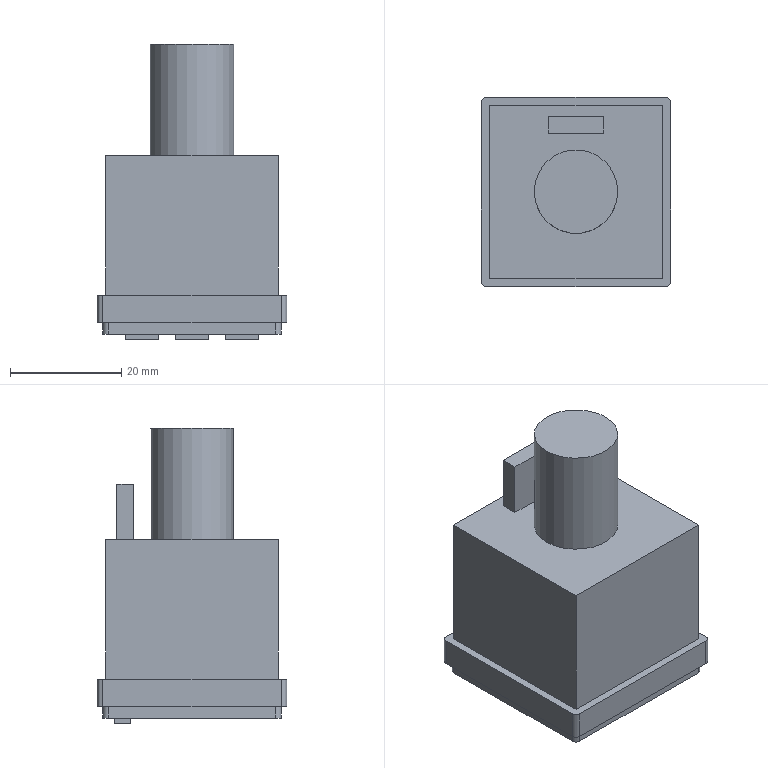Part | NX | 1 solid | 51 faces | box 34 x 34 x 53 mm | volume 35678 mm3 | plane 42 | cylinder 9 | commonest cylinder face diameters 2 x8 15 x1
STEP:
#1=CARTESIAN_POINT('',(-7.5,0.,30.));
#2=VERTEX_POINT('',#1);
#3=CARTESIAN_POINT('',(0.,0.,30.));
#4=DIRECTION('',(0.,0.,-1.));
#5=DIRECTION('',(-1.,0.,0.));
#6=AXIS2_PLACEMENT_3D('',#3,#4,#5);
#7=CIRCLE('',#6,7.5);
#8=EDGE_CURVE('',#2,#2,#7,.F.);
#9=ORIENTED_EDGE('',*,*,#8,.F.);
#10=EDGE_LOOP('',(#9));
#11=FACE_BOUND('',#10,.T.);
#12=CARTESIAN_POINT('',(-15.5,15.5,30.));
#13=VERTEX_POINT('',#12);
#14=CARTESIAN_POINT('',(-15.5,-15.5,30.));
#15=VERTEX_POINT('',#14);
#16=CARTESIAN_POINT('',(-15.5,15.5,30.));
#17=DIRECTION('',(0.,-1.,0.));
#18=VECTOR('',#17,1000.);
#19=LINE('',#16,#18);
#20=EDGE_CURVE('',#13,#15,#19,.T.);
#21=ORIENTED_EDGE('',*,*,#20,.T.);
#22=CARTESIAN_POINT('',(15.5,-15.5,30.));
#23=VERTEX_POINT('',#22);
#24=CARTESIAN_POINT('',(15.5,-15.5,30.));
#25=DIRECTION('',(1.,0.,0.));
#26=VECTOR('',#25,1000.);
#27=LINE('',#24,#26);
#28=EDGE_CURVE('',#15,#23,#27,.T.);
#29=ORIENTED_EDGE('',*,*,#28,.T.);
#30=CARTESIAN_POINT('',(15.5,15.5,30.));
#31=VERTEX_POINT('',#30);
#32=CARTESIAN_POINT('',(15.5,15.5,30.));
#33=DIRECTION('',(0.,1.,0.));
#34=VECTOR('',#33,1000.);
#35=LINE('',#32,#34);
#36=EDGE_CURVE('',#23,#31,#35,.T.);
#37=ORIENTED_EDGE('',*,*,#36,.T.);
#38=CARTESIAN_POINT('',(15.5,15.5,30.));
#39=DIRECTION('',(-1.,0.,0.));
#40=VECTOR('',#39,1000.);
#41=LINE('',#38,#40);
#42=EDGE_CURVE('',#31,#13,#41,.T.);
#43=ORIENTED_EDGE('',*,*,#42,.T.);
#44=EDGE_LOOP('',(#21,#29,#37,#43));
#45=FACE_BOUND('',#44,.T.);
#46=CARTESIAN_POINT('',(5.,10.5,30.));
#47=VERTEX_POINT('',#46);
#48=CARTESIAN_POINT('',(5.,13.5,30.));
#49=VERTEX_POINT('',#48);
#50=CARTESIAN_POINT('',(5.,13.5,30.));
#51=DIRECTION('',(0.,1.,0.));
#52=VECTOR('',#51,1000.);
#53=LINE('',#50,#52);
#54=EDGE_CURVE('',#47,#49,#53,.T.);
#55=ORIENTED_EDGE('',*,*,#54,.F.);
#56=CARTESIAN_POINT('',(-5.,10.5,30.));
#57=VERTEX_POINT('',#56);
#58=CARTESIAN_POINT('',(5.,10.5,30.));
#59=DIRECTION('',(1.,0.,0.));
#60=VECTOR('',#59,1000.);
#61=LINE('',#58,#60);
#62=EDGE_CURVE('',#57,#47,#61,.T.);
#63=ORIENTED_EDGE('',*,*,#62,.F.);
#64=CARTESIAN_POINT('',(-5.,13.5,30.));
#65=VERTEX_POINT('',#64);
#66=CARTESIAN_POINT('',(-5.,13.5,30.));
#67=DIRECTION('',(0.,-1.,0.));
#68=VECTOR('',#67,1000.);
#69=LINE('',#66,#68);
#70=EDGE_CURVE('',#65,#57,#69,.T.);
#71=ORIENTED_EDGE('',*,*,#70,.F.);
#72=CARTESIAN_POINT('',(5.,13.5,30.));
#73=DIRECTION('',(-1.,0.,0.));
#74=VECTOR('',#73,1000.);
#75=LINE('',#72,#74);
#76=EDGE_CURVE('',#49,#65,#75,.T.);
#77=ORIENTED_EDGE('',*,*,#76,.F.);
#78=EDGE_LOOP('',(#55,#63,#71,#77));
#79=FACE_BOUND('',#78,.T.);
#80=CARTESIAN_POINT('',(0.,0.,30.));
#81=DIRECTION('',(0.,0.,-1.));
#82=DIRECTION('',(-1.,0.,0.));
#83=AXIS2_PLACEMENT_3D('',#80,#81,#82);
#84=PLANE('',#83);
#85=ADVANCED_FACE('',(#11,#45,#79),#84,.F.);
#86=CARTESIAN_POINT('',(13.,8.5,-2.));
#87=VERTEX_POINT('',#86);
#88=CARTESIAN_POINT('',(13.,-13.5,-2.));
#89=VERTEX_POINT('',#88);
#90=CARTESIAN_POINT('',(13.,8.5,-2.));
#91=DIRECTION('',(0.,-1.,0.));
#92=VECTOR('',#91,1000.);
#93=LINE('',#90,#92);
#94=EDGE_CURVE('',#87,#89,#93,.T.);
#95=ORIENTED_EDGE('',*,*,#94,.F.);
#96=CARTESIAN_POINT('',(-13.,8.5,-2.));
#97=VERTEX_POINT('',#96);
#98=CARTESIAN_POINT('',(-13.,8.5,-2.));
#99=DIRECTION('',(1.,0.,0.));
#100=VECTOR('',#99,1000.);
#101=LINE('',#98,#100);
#102=EDGE_CURVE('',#97,#87,#101,.T.);
#103=ORIENTED_EDGE('',*,*,#102,.F.);
#104=CARTESIAN_POINT('',(-13.,-13.5,-2.));
#105=VERTEX_POINT('',#104);
#106=CARTESIAN_POINT('',(-13.,8.5,-2.));
#107=DIRECTION('',(0.,1.,0.));
#108=VECTOR('',#107,1000.);
#109=LINE('',#106,#108);
#110=EDGE_CURVE('',#105,#97,#109,.T.);
#111=ORIENTED_EDGE('',*,*,#110,.F.);
#112=CARTESIAN_POINT('',(-13.,-13.5,-2.));
#113=DIRECTION('',(-1.,0.,0.));
#114=VECTOR('',#113,1000.);
#115=LINE('',#112,#114);
#116=EDGE_CURVE('',#89,#105,#115,.T.);
#117=ORIENTED_EDGE('',*,*,#116,.F.);
#118=EDGE_LOOP('',(#95,#103,#111,#117));
#119=FACE_BOUND('',#118,.T.);
#120=CARTESIAN_POINT('',(3.,11.,-2.));
#121=VERTEX_POINT('',#120);
#122=CARTESIAN_POINT('',(-3.,11.,-2.));
#123=VERTEX_POINT('',#122);
#124=CARTESIAN_POINT('',(3.,11.,-2.));
#125=DIRECTION('',(-1.,0.,0.));
#126=VECTOR('',#125,1000.);
#127=LINE('',#124,#126);
#128=EDGE_CURVE('',#121,#123,#127,.T.);
#129=ORIENTED_EDGE('',*,*,#128,.F.);
#130=CARTESIAN_POINT('',(3.,14.,-2.));
#131=VERTEX_POINT('',#130);
#132=CARTESIAN_POINT('',(3.,14.,-2.));
#133=DIRECTION('',(0.,-1.,0.));
#134=VECTOR('',#133,1000.);
#135=LINE('',#132,#134);
#136=EDGE_CURVE('',#131,#121,#135,.T.);
#137=ORIENTED_EDGE('',*,*,#136,.F.);
#138=CARTESIAN_POINT('',(-3.,14.,-2.));
#139=VERTEX_POINT('',#138);
#140=CARTESIAN_POINT('',(3.,14.,-2.));
#141=DIRECTION('',(1.,0.,0.));
#142=VECTOR('',#141,1000.);
#143=LINE('',#140,#142);
#144=EDGE_CURVE('',#139,#131,#143,.T.);
#145=ORIENTED_EDGE('',*,*,#144,.F.);
#146=CARTESIAN_POINT('',(-3.,14.,-2.));
#147=DIRECTION('',(0.,1.,0.));
#148=VECTOR('',#147,1000.);
#149=LINE('',#146,#148);
#150=EDGE_CURVE('',#123,#139,#149,.T.);
#151=ORIENTED_EDGE('',*,*,#150,.F.);
#152=EDGE_LOOP('',(#129,#137,#145,#151));
#153=FACE_BOUND('',#152,.T.);
#154=CARTESIAN_POINT('',(-15.,16.,-2.));
#155=VERTEX_POINT('',#154);
#156=CARTESIAN_POINT('',(15.,16.,-2.));
#157=VERTEX_POINT('',#156);
#158=CARTESIAN_POINT('',(-16.,16.,-2.));
#159=DIRECTION('',(1.,0.,0.));
#160=VECTOR('',#159,1000.);
#161=LINE('',#158,#160);
#162=EDGE_CURVE('',#155,#157,#161,.T.);
#163=ORIENTED_EDGE('',*,*,#162,.T.);
#164=CARTESIAN_POINT('',(16.,15.,-2.));
#165=VERTEX_POINT('',#164);
#166=CARTESIAN_POINT('',(15.,15.,-2.));
#167=DIRECTION('',(0.,0.,-1.));
#168=DIRECTION('',(-1.,0.,0.));
#169=AXIS2_PLACEMENT_3D('',#166,#167,#168);
#170=CIRCLE('',#169,1.);
#171=EDGE_CURVE('',#157,#165,#170,.T.);
#172=ORIENTED_EDGE('',*,*,#171,.T.);
#173=CARTESIAN_POINT('',(16.,-15.,-2.));
#174=VERTEX_POINT('',#173);
#175=CARTESIAN_POINT('',(16.,16.,-2.));
#176=DIRECTION('',(0.,-1.,0.));
#177=VECTOR('',#176,1000.);
#178=LINE('',#175,#177);
#179=EDGE_CURVE('',#165,#174,#178,.T.);
#180=ORIENTED_EDGE('',*,*,#179,.T.);
#181=CARTESIAN_POINT('',(15.,-16.,-2.));
#182=VERTEX_POINT('',#181);
#183=CARTESIAN_POINT('',(15.,-15.,-2.));
#184=DIRECTION('',(0.,0.,-1.));
#185=DIRECTION('',(-1.,0.,0.));
#186=AXIS2_PLACEMENT_3D('',#183,#184,#185);
#187=CIRCLE('',#186,1.);
#188=EDGE_CURVE('',#174,#182,#187,.T.);
#189=ORIENTED_EDGE('',*,*,#188,.T.);
#190=CARTESIAN_POINT('',(-15.,-16.,-2.));
#191=VERTEX_POINT('',#190);
#192=CARTESIAN_POINT('',(16.,-16.,-2.));
#193=DIRECTION('',(-1.,0.,0.));
#194=VECTOR('',#193,1000.);
#195=LINE('',#192,#194);
#196=EDGE_CURVE('',#182,#191,#195,.T.);
#197=ORIENTED_EDGE('',*,*,#196,.T.);
#198=CARTESIAN_POINT('',(-16.,-15.,-2.));
#199=VERTEX_POINT('',#198);
#200=CARTESIAN_POINT('',(-15.,-15.,-2.));
#201=DIRECTION('',(0.,0.,-1.));
#202=DIRECTION('',(-1.,0.,0.));
#203=AXIS2_PLACEMENT_3D('',#200,#201,#202);
#204=CIRCLE('',#203,1.);
#205=EDGE_CURVE('',#191,#199,#204,.T.);
#206=ORIENTED_EDGE('',*,*,#205,.T.);
#207=CARTESIAN_POINT('',(-16.,15.,-2.));
#208=VERTEX_POINT('',#207);
#209=CARTESIAN_POINT('',(-16.,-16.,-2.));
#210=DIRECTION('',(0.,1.,0.));
#211=VECTOR('',#210,1000.);
#212=LINE('',#209,#211);
#213=EDGE_CURVE('',#199,#208,#212,.T.);
#214=ORIENTED_EDGE('',*,*,#213,.T.);
#215=CARTESIAN_POINT('',(-15.,15.,-2.));
#216=DIRECTION('',(0.,0.,-1.));
#217=DIRECTION('',(-1.,0.,0.));
#218=AXIS2_PLACEMENT_3D('',#215,#216,#217);
#219=CIRCLE('',#218,1.);
#220=EDGE_CURVE('',#208,#155,#219,.T.);
#221=ORIENTED_EDGE('',*,*,#220,.T.);
#222=EDGE_LOOP('',(#163,#172,#180,#189,#197,#206,#214,#221));
#223=FACE_BOUND('',#222,.T.);
#224=CARTESIAN_POINT('',(12.,11.,-2.));
#225=VERTEX_POINT('',#224);
#226=CARTESIAN_POINT('',(6.,11.,-2.));
#227=VERTEX_POINT('',#226);
#228=CARTESIAN_POINT('',(12.,11.,-2.));
#229=DIRECTION('',(-1.,0.,0.));
#230=VECTOR('',#229,1000.);
#231=LINE('',#228,#230);
#232=EDGE_CURVE('',#225,#227,#231,.T.);
#233=ORIENTED_EDGE('',*,*,#232,.F.);
#234=CARTESIAN_POINT('',(12.,14.,-2.));
#235=VERTEX_POINT('',#234);
#236=CARTESIAN_POINT('',(12.,14.,-2.));
#237=DIRECTION('',(0.,-1.,0.));
#238=VECTOR('',#237,1000.);
#239=LINE('',#236,#238);
#240=EDGE_CURVE('',#235,#225,#239,.T.);
#241=ORIENTED_EDGE('',*,*,#240,.F.);
#242=CARTESIAN_POINT('',(6.,14.,-2.));
#243=VERTEX_POINT('',#242);
#244=CARTESIAN_POINT('',(12.,14.,-2.));
#245=DIRECTION('',(1.,0.,0.));
#246=VECTOR('',#245,1000.);
#247=LINE('',#244,#246);
#248=EDGE_CURVE('',#243,#235,#247,.T.);
#249=ORIENTED_EDGE('',*,*,#248,.F.);
#250=CARTESIAN_POINT('',(6.,14.,-2.));
#251=DIRECTION('',(0.,1.,0.));
#252=VECTOR('',#251,1000.);
#253=LINE('',#250,#252);
#254=EDGE_CURVE('',#227,#243,#253,.T.);
#255=ORIENTED_EDGE('',*,*,#254,.F.);
#256=EDGE_LOOP('',(#233,#241,#249,#255));
#257=FACE_BOUND('',#256,.T.);
#258=CARTESIAN_POINT('',(-6.,11.,-2.));
#259=VERTEX_POINT('',#258);
#260=CARTESIAN_POINT('',(-12.,11.,-2.));
#261=VERTEX_POINT('',#260);
#262=CARTESIAN_POINT('',(-6.,11.,-2.));
#263=DIRECTION('',(-1.,0.,0.));
#264=VECTOR('',#263,1000.);
#265=LINE('',#262,#264);
#266=EDGE_CURVE('',#259,#261,#265,.T.);
#267=ORIENTED_EDGE('',*,*,#266,.F.);
#268=CARTESIAN_POINT('',(-6.,14.,-2.));
#269=VERTEX_POINT('',#268);
#270=CARTESIAN_POINT('',(-6.,14.,-2.));
#271=DIRECTION('',(0.,-1.,0.));
#272=VECTOR('',#271,1000.);
#273=LINE('',#270,#272);
#274=EDGE_CURVE('',#269,#259,#273,.T.);
#275=ORIENTED_EDGE('',*,*,#274,.F.);
#276=CARTESIAN_POINT('',(-12.,14.,-2.));
#277=VERTEX_POINT('',#276);
#278=CARTESIAN_POINT('',(-6.,14.,-2.));
#279=DIRECTION('',(1.,0.,0.));
#280=VECTOR('',#279,1000.);
#281=LINE('',#278,#280);
#282=EDGE_CURVE('',#277,#269,#281,.T.);
#283=ORIENTED_EDGE('',*,*,#282,.F.);
#284=CARTESIAN_POINT('',(-12.,14.,-2.));
#285=DIRECTION('',(0.,1.,0.));
#286=VECTOR('',#285,1000.);
#287=LINE('',#284,#286);
#288=EDGE_CURVE('',#261,#277,#287,.T.);
#289=ORIENTED_EDGE('',*,*,#288,.F.);
#290=EDGE_LOOP('',(#267,#275,#283,#289));
#291=FACE_BOUND('',#290,.T.);
#292=CARTESIAN_POINT('',(0.,0.,-2.));
#293=DIRECTION('',(0.,0.,-1.));
#294=DIRECTION('',(-1.,0.,0.));
#295=AXIS2_PLACEMENT_3D('',#292,#293,#294);
#296=PLANE('',#295);
#297=ADVANCED_FACE('',(#119,#153,#223,#257,#291),#296,.T.);
#298=CARTESIAN_POINT('',(16.,17.,0.));
#299=VERTEX_POINT('',#298);
#300=CARTESIAN_POINT('',(-16.,17.,0.));
#301=VERTEX_POINT('',#300);
#302=CARTESIAN_POINT('',(-17.,17.,0.));
#303=DIRECTION('',(-1.,0.,0.));
#304=VECTOR('',#303,1000.);
#305=LINE('',#302,#304);
#306=EDGE_CURVE('',#299,#301,#305,.T.);
#307=ORIENTED_EDGE('',*,*,#306,.F.);
#308=CARTESIAN_POINT('',(17.,16.,0.));
#309=VERTEX_POINT('',#308);
#310=CARTESIAN_POINT('',(16.,16.,0.));
#311=DIRECTION('',(0.,0.,1.));
#312=DIRECTION('',(1.,0.,0.));
#313=AXIS2_PLACEMENT_3D('',#310,#311,#312);
#314=CIRCLE('',#313,1.);
#315=EDGE_CURVE('',#299,#309,#314,.F.);
#316=ORIENTED_EDGE('',*,*,#315,.T.);
#317=CARTESIAN_POINT('',(17.,-16.,0.));
#318=VERTEX_POINT('',#317);
#319=CARTESIAN_POINT('',(17.,17.,0.));
#320=DIRECTION('',(0.,1.,0.));
#321=VECTOR('',#320,1000.);
#322=LINE('',#319,#321);
#323=EDGE_CURVE('',#318,#309,#322,.T.);
#324=ORIENTED_EDGE('',*,*,#323,.F.);
#325=CARTESIAN_POINT('',(16.,-17.,0.));
#326=VERTEX_POINT('',#325);
#327=CARTESIAN_POINT('',(16.,-16.,0.));
#328=DIRECTION('',(0.,0.,1.));
#329=DIRECTION('',(1.,0.,0.));
#330=AXIS2_PLACEMENT_3D('',#327,#328,#329);
#331=CIRCLE('',#330,1.);
#332=EDGE_CURVE('',#318,#326,#331,.F.);
#333=ORIENTED_EDGE('',*,*,#332,.T.);
#334=CARTESIAN_POINT('',(-16.,-17.,0.));
#335=VERTEX_POINT('',#334);
#336=CARTESIAN_POINT('',(-17.,-17.,0.));
#337=DIRECTION('',(1.,0.,0.));
#338=VECTOR('',#337,1000.);
#339=LINE('',#336,#338);
#340=EDGE_CURVE('',#335,#326,#339,.T.);
#341=ORIENTED_EDGE('',*,*,#340,.F.);
#342=CARTESIAN_POINT('',(-17.,-16.,0.));
#343=VERTEX_POINT('',#342);
#344=CARTESIAN_POINT('',(-16.,-16.,0.));
#345=DIRECTION('',(0.,0.,1.));
#346=DIRECTION('',(1.,0.,0.));
#347=AXIS2_PLACEMENT_3D('',#344,#345,#346);
#348=CIRCLE('',#347,1.);
#349=EDGE_CURVE('',#335,#343,#348,.F.);
#350=ORIENTED_EDGE('',*,*,#349,.T.);
#351=CARTESIAN_POINT('',(-17.,16.,0.));
#352=VERTEX_POINT('',#351);
#353=CARTESIAN_POINT('',(-17.,17.,0.));
#354=DIRECTION('',(0.,-1.,0.));
#355=VECTOR('',#354,1000.);
#356=LINE('',#353,#355);
#357=EDGE_CURVE('',#352,#343,#356,.T.);
#358=ORIENTED_EDGE('',*,*,#357,.F.);
#359=CARTESIAN_POINT('',(-16.,16.,0.));
#360=DIRECTION('',(0.,0.,1.));
#361=DIRECTION('',(1.,0.,0.));
#362=AXIS2_PLACEMENT_3D('',#359,#360,#361);
#363=CIRCLE('',#362,1.);
#364=EDGE_CURVE('',#352,#301,#363,.F.);
#365=ORIENTED_EDGE('',*,*,#364,.T.);
#366=EDGE_LOOP('',(#307,#316,#324,#333,#341,#350,#358,#365));
#367=FACE_BOUND('',#366,.T.);
#368=CARTESIAN_POINT('',(-15.,16.,0.));
#369=VERTEX_POINT('',#368);
#370=CARTESIAN_POINT('',(15.,16.,0.));
#371=VERTEX_POINT('',#370);
#372=CARTESIAN_POINT('',(-16.,16.,0.));
#373=DIRECTION('',(1.,0.,0.));
#374=VECTOR('',#373,1000.);
#375=LINE('',#372,#374);
#376=EDGE_CURVE('',#369,#371,#375,.T.);
#377=ORIENTED_EDGE('',*,*,#376,.F.);
#378=CARTESIAN_POINT('',(-16.,15.,0.));
#379=VERTEX_POINT('',#378);
#380=CARTESIAN_POINT('',(-15.,15.,0.));
#381=DIRECTION('',(0.,0.,1.));
#382=DIRECTION('',(1.,0.,0.));
#383=AXIS2_PLACEMENT_3D('',#380,#381,#382);
#384=CIRCLE('',#383,1.);
#385=EDGE_CURVE('',#369,#379,#384,.T.);
#386=ORIENTED_EDGE('',*,*,#385,.T.);
#387=CARTESIAN_POINT('',(-16.,-15.,0.));
#388=VERTEX_POINT('',#387);
#389=CARTESIAN_POINT('',(-16.,-16.,0.));
#390=DIRECTION('',(0.,1.,0.));
#391=VECTOR('',#390,1000.);
#392=LINE('',#389,#391);
#393=EDGE_CURVE('',#388,#379,#392,.T.);
#394=ORIENTED_EDGE('',*,*,#393,.F.);
#395=CARTESIAN_POINT('',(-15.,-16.,0.));
#396=VERTEX_POINT('',#395);
#397=CARTESIAN_POINT('',(-15.,-15.,0.));
#398=DIRECTION('',(0.,0.,1.));
#399=DIRECTION('',(1.,0.,0.));
#400=AXIS2_PLACEMENT_3D('',#397,#398,#399);
#401=CIRCLE('',#400,1.);
#402=EDGE_CURVE('',#388,#396,#401,.T.);
#403=ORIENTED_EDGE('',*,*,#402,.T.);
#404=CARTESIAN_POINT('',(15.,-16.,0.));
#405=VERTEX_POINT('',#404);
#406=CARTESIAN_POINT('',(16.,-16.,0.));
#407=DIRECTION('',(-1.,0.,0.));
#408=VECTOR('',#407,1000.);
#409=LINE('',#406,#408);
#410=EDGE_CURVE('',#405,#396,#409,.T.);
#411=ORIENTED_EDGE('',*,*,#410,.F.);
#412=CARTESIAN_POINT('',(16.,-15.,0.));
#413=VERTEX_POINT('',#412);
#414=CARTESIAN_POINT('',(15.,-15.,0.));
#415=DIRECTION('',(0.,0.,1.));
#416=DIRECTION('',(1.,0.,0.));
#417=AXIS2_PLACEMENT_3D('',#414,#415,#416);
#418=CIRCLE('',#417,1.);
#419=EDGE_CURVE('',#405,#413,#418,.T.);
#420=ORIENTED_EDGE('',*,*,#419,.T.);
#421=CARTESIAN_POINT('',(16.,15.,0.));
#422=VERTEX_POINT('',#421);
#423=CARTESIAN_POINT('',(16.,16.,0.));
#424=DIRECTION('',(0.,-1.,0.));
#425=VECTOR('',#424,1000.);
#426=LINE('',#423,#425);
#427=EDGE_CURVE('',#422,#413,#426,.T.);
#428=ORIENTED_EDGE('',*,*,#427,.F.);
#429=CARTESIAN_POINT('',(15.,15.,0.));
#430=DIRECTION('',(0.,0.,1.));
#431=DIRECTION('',(1.,0.,0.));
#432=AXIS2_PLACEMENT_3D('',#429,#430,#431);
#433=CIRCLE('',#432,1.);
#434=EDGE_CURVE('',#422,#371,#433,.T.);
#435=ORIENTED_EDGE('',*,*,#434,.T.);
#436=EDGE_LOOP('',(#377,#386,#394,#403,#411,#420,#428,#435));
#437=FACE_BOUND('',#436,.T.);
#438=CARTESIAN_POINT('',(0.,0.,0.));
#439=DIRECTION('',(0.,0.,1.));
#440=DIRECTION('',(1.,0.,0.));
#441=AXIS2_PLACEMENT_3D('',#438,#439,#440);
#442=PLANE('',#441);
#443=ADVANCED_FACE('',(#367,#437),#442,.F.);
#444=CARTESIAN_POINT('',(17.,-16.,5.));
#445=VERTEX_POINT('',#444);
#446=CARTESIAN_POINT('',(17.,16.,5.));
#447=VERTEX_POINT('',#446);
#448=CARTESIAN_POINT('',(17.,17.,5.));
#449=DIRECTION('',(0.,1.,0.));
#450=VECTOR('',#449,1000.);
#451=LINE('',#448,#450);
#452=EDGE_CURVE('',#445,#447,#451,.T.);
#453=ORIENTED_EDGE('',*,*,#452,.T.);
#454=CARTESIAN_POINT('',(16.,17.,5.));
#455=VERTEX_POINT('',#454);
#456=CARTESIAN_POINT('',(16.,16.,5.));
#457=DIRECTION('',(0.,0.,1.));
#458=DIRECTION('',(1.,0.,0.));
#459=AXIS2_PLACEMENT_3D('',#456,#457,#458);
#460=CIRCLE('',#459,1.);
#461=EDGE_CURVE('',#447,#455,#460,.T.);
#462=ORIENTED_EDGE('',*,*,#461,.T.);
#463=CARTESIAN_POINT('',(-16.,17.,5.));
#464=VERTEX_POINT('',#463);
#465=CARTESIAN_POINT('',(-17.,17.,5.));
#466=DIRECTION('',(-1.,0.,0.));
#467=VECTOR('',#466,1000.);
#468=LINE('',#465,#467);
#469=EDGE_CURVE('',#455,#464,#468,.T.);
#470=ORIENTED_EDGE('',*,*,#469,.T.);
#471=CARTESIAN_POINT('',(-17.,16.,5.));
#472=VERTEX_POINT('',#471);
#473=CARTESIAN_POINT('',(-16.,16.,5.));
#474=DIRECTION('',(0.,0.,1.));
#475=DIRECTION('',(1.,0.,0.));
#476=AXIS2_PLACEMENT_3D('',#473,#474,#475);
#477=CIRCLE('',#476,1.);
#478=EDGE_CURVE('',#464,#472,#477,.T.);
#479=ORIENTED_EDGE('',*,*,#478,.T.);
#480=CARTESIAN_POINT('',(-17.,-16.,5.));
#481=VERTEX_POINT('',#480);
#482=CARTESIAN_POINT('',(-17.,17.,5.));
#483=DIRECTION('',(0.,-1.,0.));
#484=VECTOR('',#483,1000.);
#485=LINE('',#482,#484);
#486=EDGE_CURVE('',#472,#481,#485,.T.);
#487=ORIENTED_EDGE('',*,*,#486,.T.);
#488=CARTESIAN_POINT('',(-16.,-17.,5.));
#489=VERTEX_POINT('',#488);
#490=CARTESIAN_POINT('',(-16.,-16.,5.));
#491=DIRECTION('',(0.,0.,1.));
#492=DIRECTION('',(1.,0.,0.));
#493=AXIS2_PLACEMENT_3D('',#490,#491,#492);
#494=CIRCLE('',#493,1.);
#495=EDGE_CURVE('',#481,#489,#494,.T.);
#496=ORIENTED_EDGE('',*,*,#495,.T.);
#497=CARTESIAN_POINT('',(16.,-17.,5.));
#498=VERTEX_POINT('',#497);
#499=CARTESIAN_POINT('',(-17.,-17.,5.));
#500=DIRECTION('',(1.,0.,0.));
#501=VECTOR('',#500,1000.);
#502=LINE('',#499,#501);
#503=EDGE_CURVE('',#489,#498,#502,.T.);
#504=ORIENTED_EDGE('',*,*,#503,.T.);
#505=CARTESIAN_POINT('',(16.,-16.,5.));
#506=DIRECTION('',(0.,0.,1.));
#507=DIRECTION('',(1.,0.,0.));
#508=AXIS2_PLACEMENT_3D('',#505,#506,#507);
#509=CIRCLE('',#508,1.);
#510=EDGE_CURVE('',#498,#445,#509,.T.);
#511=ORIENTED_EDGE('',*,*,#510,.T.);
#512=EDGE_LOOP('',(#453,#462,#470,#479,#487,#496,#504,#511));
#513=FACE_BOUND('',#512,.T.);
#514=CARTESIAN_POINT('',(-15.5,-15.5,5.));
#515=VERTEX_POINT('',#514);
#516=CARTESIAN_POINT('',(15.5,-15.5,5.));
#517=VERTEX_POINT('',#516);
#518=CARTESIAN_POINT('',(15.5,-15.5,5.));
#519=DIRECTION('',(1.,0.,0.));
#520=VECTOR('',#519,1000.);
#521=LINE('',#518,#520);
#522=EDGE_CURVE('',#515,#517,#521,.T.);
#523=ORIENTED_EDGE('',*,*,#522,.F.);
#524=CARTESIAN_POINT('',(-15.5,15.5,5.));
#525=VERTEX_POINT('',#524);
#526=CARTESIAN_POINT('',(-15.5,15.5,5.));
#527=DIRECTION('',(0.,-1.,0.));
#528=VECTOR('',#527,1000.);
#529=LINE('',#526,#528);
#530=EDGE_CURVE('',#525,#515,#529,.T.);
#531=ORIENTED_EDGE('',*,*,#530,.F.);
#532=CARTESIAN_POINT('',(15.5,15.5,5.));
#533=VERTEX_POINT('',#532);
#534=CARTESIAN_POINT('',(15.5,15.5,5.));
#535=DIRECTION('',(-1.,0.,0.));
#536=VECTOR('',#535,1000.);
#537=LINE('',#534,#536);
#538=EDGE_CURVE('',#533,#525,#537,.T.);
#539=ORIENTED_EDGE('',*,*,#538,.F.);
#540=CARTESIAN_POINT('',(15.5,15.5,5.));
#541=DIRECTION('',(0.,1.,0.));
#542=VECTOR('',#541,1000.);
#543=LINE('',#540,#542);
#544=EDGE_CURVE('',#517,#533,#543,.T.);
#545=ORIENTED_EDGE('',*,*,#544,.F.);
#546=EDGE_LOOP('',(#523,#531,#539,#545));
#547=FACE_BOUND('',#546,.T.);
#548=CARTESIAN_POINT('',(0.,0.,5.));
#549=DIRECTION('',(0.,0.,1.));
#550=DIRECTION('',(1.,0.,0.));
#551=AXIS2_PLACEMENT_3D('',#548,#549,#550);
#552=PLANE('',#551);
#553=ADVANCED_FACE('',(#513,#547),#552,.T.);
#554=ORIENTED_EDGE('',*,*,#323,.T.);
#555=CARTESIAN_POINT('',(17.,16.,5.));
#556=DIRECTION('',(0.,0.,-1.));
#557=VECTOR('',#556,1000.);
#558=LINE('',#555,#557);
#559=EDGE_CURVE('',#309,#447,#558,.F.);
#560=ORIENTED_EDGE('',*,*,#559,.T.);
#561=ORIENTED_EDGE('',*,*,#452,.F.);
#562=CARTESIAN_POINT('',(17.,-16.,5.));
#563=DIRECTION('',(0.,0.,-1.));
#564=VECTOR('',#563,1000.);
#565=LINE('',#562,#564);
#566=EDGE_CURVE('',#445,#318,#565,.T.);
#567=ORIENTED_EDGE('',*,*,#566,.T.);
#568=EDGE_LOOP('',(#554,#560,#561,#567));
#569=FACE_BOUND('',#568,.T.);
#570=CARTESIAN_POINT('',(17.,17.,5.));
#571=DIRECTION('',(-1.,0.,0.));
#572=DIRECTION('',(0.,-1.,0.));
#573=AXIS2_PLACEMENT_3D('',#570,#571,#572);
#574=PLANE('',#573);
#575=ADVANCED_FACE('',(#569),#574,.F.);
#576=ORIENTED_EDGE('',*,*,#469,.F.);
#577=CARTESIAN_POINT('',(16.,17.,5.));
#578=DIRECTION('',(0.,0.,-1.));
#579=VECTOR('',#578,1000.);
#580=LINE('',#577,#579);
#581=EDGE_CURVE('',#455,#299,#580,.T.);
#582=ORIENTED_EDGE('',*,*,#581,.T.);
#583=ORIENTED_EDGE('',*,*,#306,.T.);
#584=CARTESIAN_POINT('',(-16.,17.,5.));
#585=DIRECTION('',(0.,0.,-1.));
#586=VECTOR('',#585,1000.);
#587=LINE('',#584,#586);
#588=EDGE_CURVE('',#301,#464,#587,.F.);
#589=ORIENTED_EDGE('',*,*,#588,.T.);
#590=EDGE_LOOP('',(#576,#582,#583,#589));
#591=FACE_BOUND('',#590,.T.);
#592=CARTESIAN_POINT('',(-17.,17.,5.));
#593=DIRECTION('',(0.,-1.,0.));
#594=DIRECTION('',(0.,0.,-1.));
#595=AXIS2_PLACEMENT_3D('',#592,#593,#594);
#596=PLANE('',#595);
#597=ADVANCED_FACE('',(#591),#596,.F.);
#598=ORIENTED_EDGE('',*,*,#486,.F.);
#599=CARTESIAN_POINT('',(-17.,16.,5.));
#600=DIRECTION('',(0.,0.,-1.));
#601=VECTOR('',#600,1000.);
#602=LINE('',#599,#601);
#603=EDGE_CURVE('',#472,#352,#602,.T.);
#604=ORIENTED_EDGE('',*,*,#603,.T.);
#605=ORIENTED_EDGE('',*,*,#357,.T.);
#606=CARTESIAN_POINT('',(-17.,-16.,5.));
#607=DIRECTION('',(0.,0.,-1.));
#608=VECTOR('',#607,1000.);
#609=LINE('',#606,#608);
#610=EDGE_CURVE('',#343,#481,#609,.F.);
#611=ORIENTED_EDGE('',*,*,#610,.T.);
#612=EDGE_LOOP('',(#598,#604,#605,#611));
#613=FACE_BOUND('',#612,.T.);
#614=CARTESIAN_POINT('',(-17.,17.,5.));
#615=DIRECTION('',(1.,0.,0.));
#616=DIRECTION('',(0.,1.,0.));
#617=AXIS2_PLACEMENT_3D('',#614,#615,#616);
#618=PLANE('',#617);
#619=ADVANCED_FACE('',(#613),#618,.F.);
#620=ORIENTED_EDGE('',*,*,#503,.F.);
#621=CARTESIAN_POINT('',(-16.,-17.,5.));
#622=DIRECTION('',(0.,0.,-1.));
#623=VECTOR('',#622,1000.);
#624=LINE('',#621,#623);
#625=EDGE_CURVE('',#489,#335,#624,.T.);
#626=ORIENTED_EDGE('',*,*,#625,.T.);
#627=ORIENTED_EDGE('',*,*,#340,.T.);
#628=CARTESIAN_POINT('',(16.,-17.,5.));
#629=DIRECTION('',(0.,0.,-1.));
#630=VECTOR('',#629,1000.);
#631=LINE('',#628,#630);
#632=EDGE_CURVE('',#326,#498,#631,.F.);
#633=ORIENTED_EDGE('',*,*,#632,.T.);
#634=EDGE_LOOP('',(#620,#626,#627,#633));
#635=FACE_BOUND('',#634,.T.);
#636=CARTESIAN_POINT('',(-17.,-17.,5.));
#637=DIRECTION('',(0.,1.,0.));
#638=DIRECTION('',(0.,0.,1.));
#639=AXIS2_PLACEMENT_3D('',#636,#637,#638);
#640=PLANE('',#639);
#641=ADVANCED_FACE('',(#635),#640,.F.);
#642=ORIENTED_EDGE('',*,*,#530,.T.);
#643=CARTESIAN_POINT('',(-15.5,-15.5,30.));
#644=DIRECTION('',(0.,0.,-1.));
#645=VECTOR('',#644,1000.);
#646=LINE('',#643,#645);
#647=EDGE_CURVE('',#15,#515,#646,.T.);
#648=ORIENTED_EDGE('',*,*,#647,.F.);
#649=ORIENTED_EDGE('',*,*,#20,.F.);
#650=CARTESIAN_POINT('',(-15.5,15.5,30.));
#651=DIRECTION('',(0.,0.,-1.));
#652=VECTOR('',#651,1000.);
#653=LINE('',#650,#652);
#654=EDGE_CURVE('',#13,#525,#653,.T.);
#655=ORIENTED_EDGE('',*,*,#654,.T.);
#656=EDGE_LOOP('',(#642,#648,#649,#655));
#657=FACE_BOUND('',#656,.T.);
#658=CARTESIAN_POINT('',(-15.5,15.5,30.));
#659=DIRECTION('',(1.,0.,0.));
#660=DIRECTION('',(0.,1.,0.));
#661=AXIS2_PLACEMENT_3D('',#658,#659,#660);
#662=PLANE('',#661);
#663=ADVANCED_FACE('',(#657),#662,.F.);
#664=ORIENTED_EDGE('',*,*,#522,.T.);
#665=CARTESIAN_POINT('',(15.5,-15.5,30.));
#666=DIRECTION('',(0.,0.,-1.));
#667=VECTOR('',#666,1000.);
#668=LINE('',#665,#667);
#669=EDGE_CURVE('',#23,#517,#668,.T.);
#670=ORIENTED_EDGE('',*,*,#669,.F.);
#671=ORIENTED_EDGE('',*,*,#28,.F.);
#672=ORIENTED_EDGE('',*,*,#647,.T.);
#673=EDGE_LOOP('',(#664,#670,#671,#672));
#674=FACE_BOUND('',#673,.T.);
#675=CARTESIAN_POINT('',(15.5,-15.5,30.));
#676=DIRECTION('',(0.,1.,0.));
#677=DIRECTION('',(-1.,0.,0.));
#678=AXIS2_PLACEMENT_3D('',#675,#676,#677);
#679=PLANE('',#678);
#680=ADVANCED_FACE('',(#674),#679,.F.);
#681=ORIENTED_EDGE('',*,*,#544,.T.);
#682=CARTESIAN_POINT('',(15.5,15.5,30.));
#683=DIRECTION('',(0.,0.,-1.));
#684=VECTOR('',#683,1000.);
#685=LINE('',#682,#684);
#686=EDGE_CURVE('',#31,#533,#685,.T.);
#687=ORIENTED_EDGE('',*,*,#686,.F.);
#688=ORIENTED_EDGE('',*,*,#36,.F.);
#689=ORIENTED_EDGE('',*,*,#669,.T.);
#690=EDGE_LOOP('',(#681,#687,#688,#689));
#691=FACE_BOUND('',#690,.T.);
#692=CARTESIAN_POINT('',(15.5,15.5,30.));
#693=DIRECTION('',(-1.,0.,0.));
#694=DIRECTION('',(0.,-1.,0.));
#695=AXIS2_PLACEMENT_3D('',#692,#693,#694);
#696=PLANE('',#695);
#697=ADVANCED_FACE('',(#691),#696,.F.);
#698=ORIENTED_EDGE('',*,*,#538,.T.);
#699=ORIENTED_EDGE('',*,*,#654,.F.);
#700=ORIENTED_EDGE('',*,*,#42,.F.);
#701=ORIENTED_EDGE('',*,*,#686,.T.);
#702=EDGE_LOOP('',(#698,#699,#700,#701));
#703=FACE_BOUND('',#702,.T.);
#704=CARTESIAN_POINT('',(15.5,15.5,30.));
#705=DIRECTION('',(0.,-1.,0.));
#706=DIRECTION('',(1.,0.,0.));
#707=AXIS2_PLACEMENT_3D('',#704,#705,#706);
#708=PLANE('',#707);
#709=ADVANCED_FACE('',(#703),#708,.F.);
#710=CARTESIAN_POINT('',(7.5,0.,50.));
#711=VERTEX_POINT('',#710);
#712=CARTESIAN_POINT('',(0.,0.,50.));
#713=DIRECTION('',(0.,0.,1.));
#714=DIRECTION('',(1.,0.,0.));
#715=AXIS2_PLACEMENT_3D('',#712,#713,#714);
#716=CIRCLE('',#715,7.5);
#717=EDGE_CURVE('',#711,#711,#716,.T.);
#718=ORIENTED_EDGE('',*,*,#717,.F.);
#719=EDGE_LOOP('',(#718));
#720=FACE_BOUND('',#719,.T.);
#721=ORIENTED_EDGE('',*,*,#8,.T.);
#722=EDGE_LOOP('',(#721));
#723=FACE_BOUND('',#722,.T.);
#724=CARTESIAN_POINT('',(0.,0.,50.));
#725=DIRECTION('',(0.,0.,-1.));
#726=DIRECTION('',(-1.,0.,0.));
#727=AXIS2_PLACEMENT_3D('',#724,#725,#726);
#728=CYLINDRICAL_SURFACE('',#727,7.5);
#729=ADVANCED_FACE('',(#720,#723),#728,.T.);
#730=ORIENTED_EDGE('',*,*,#717,.T.);
#731=EDGE_LOOP('',(#730));
#732=FACE_BOUND('',#731,.T.);
#733=CARTESIAN_POINT('',(0.,0.,50.));
#734=DIRECTION('',(0.,0.,1.));
#735=DIRECTION('',(1.,0.,0.));
#736=AXIS2_PLACEMENT_3D('',#733,#734,#735);
#737=PLANE('',#736);
#738=ADVANCED_FACE('',(#732),#737,.T.);
#739=ORIENTED_EDGE('',*,*,#376,.T.);
#740=CARTESIAN_POINT('',(15.,16.,-2.));
#741=DIRECTION('',(0.,0.,1.));
#742=VECTOR('',#741,1000.);
#743=LINE('',#740,#742);
#744=EDGE_CURVE('',#371,#157,#743,.F.);
#745=ORIENTED_EDGE('',*,*,#744,.T.);
#746=ORIENTED_EDGE('',*,*,#162,.F.);
#747=CARTESIAN_POINT('',(-15.,16.,-2.));
#748=DIRECTION('',(0.,0.,1.));
#749=VECTOR('',#748,1000.);
#750=LINE('',#747,#749);
#751=EDGE_CURVE('',#155,#369,#750,.T.);
#752=ORIENTED_EDGE('',*,*,#751,.T.);
#753=EDGE_LOOP('',(#739,#745,#746,#752));
#754=FACE_BOUND('',#753,.T.);
#755=CARTESIAN_POINT('',(-16.,16.,-2.));
#756=DIRECTION('',(0.,-1.,0.));
#757=DIRECTION('',(0.,0.,-1.));
#758=AXIS2_PLACEMENT_3D('',#755,#756,#757);
#759=PLANE('',#758);
#760=ADVANCED_FACE('',(#754),#759,.F.);
#761=ORIENTED_EDGE('',*,*,#179,.F.);
#762=CARTESIAN_POINT('',(16.,15.,-2.));
#763=DIRECTION('',(0.,0.,1.));
#764=VECTOR('',#763,1000.);
#765=LINE('',#762,#764);
#766=EDGE_CURVE('',#165,#422,#765,.T.);
#767=ORIENTED_EDGE('',*,*,#766,.T.);
#768=ORIENTED_EDGE('',*,*,#427,.T.);
#769=CARTESIAN_POINT('',(16.,-15.,-2.));
#770=DIRECTION('',(0.,0.,1.));
#771=VECTOR('',#770,1000.);
#772=LINE('',#769,#771);
#773=EDGE_CURVE('',#413,#174,#772,.F.);
#774=ORIENTED_EDGE('',*,*,#773,.T.);
#775=EDGE_LOOP('',(#761,#767,#768,#774));
#776=FACE_BOUND('',#775,.T.);
#777=CARTESIAN_POINT('',(16.,16.,-2.));
#778=DIRECTION('',(-1.,0.,0.));
#779=DIRECTION('',(0.,-1.,0.));
#780=AXIS2_PLACEMENT_3D('',#777,#778,#779);
#781=PLANE('',#780);
#782=ADVANCED_FACE('',(#776),#781,.F.);
#783=ORIENTED_EDGE('',*,*,#410,.T.);
#784=CARTESIAN_POINT('',(-15.,-16.,-2.));
#785=DIRECTION('',(0.,0.,1.));
#786=VECTOR('',#785,1000.);
#787=LINE('',#784,#786);
#788=EDGE_CURVE('',#396,#191,#787,.F.);
#789=ORIENTED_EDGE('',*,*,#788,.T.);
#790=ORIENTED_EDGE('',*,*,#196,.F.);
#791=CARTESIAN_POINT('',(15.,-16.,-2.));
#792=DIRECTION('',(0.,0.,1.));
#793=VECTOR('',#792,1000.);
#794=LINE('',#791,#793);
#795=EDGE_CURVE('',#182,#405,#794,.T.);
#796=ORIENTED_EDGE('',*,*,#795,.T.);
#797=EDGE_LOOP('',(#783,#789,#790,#796));
#798=FACE_BOUND('',#797,.T.);
#799=CARTESIAN_POINT('',(16.,-16.,-2.));
#800=DIRECTION('',(0.,1.,0.));
#801=DIRECTION('',(0.,0.,1.));
#802=AXIS2_PLACEMENT_3D('',#799,#800,#801);
#803=PLANE('',#802);
#804=ADVANCED_FACE('',(#798),#803,.F.);
#805=ORIENTED_EDGE('',*,*,#393,.T.);
#806=CARTESIAN_POINT('',(-16.,15.,-2.));
#807=DIRECTION('',(0.,0.,1.));
#808=VECTOR('',#807,1000.);
#809=LINE('',#806,#808);
#810=EDGE_CURVE('',#379,#208,#809,.F.);
#811=ORIENTED_EDGE('',*,*,#810,.T.);
#812=ORIENTED_EDGE('',*,*,#213,.F.);
#813=CARTESIAN_POINT('',(-16.,-15.,-2.));
#814=DIRECTION('',(0.,0.,1.));
#815=VECTOR('',#814,1000.);
#816=LINE('',#813,#815);
#817=EDGE_CURVE('',#199,#388,#816,.T.);
#818=ORIENTED_EDGE('',*,*,#817,.T.);
#819=EDGE_LOOP('',(#805,#811,#812,#818));
#820=FACE_BOUND('',#819,.T.);
#821=CARTESIAN_POINT('',(-16.,-16.,-2.));
#822=DIRECTION('',(1.,0.,0.));
#823=DIRECTION('',(0.,1.,0.));
#824=AXIS2_PLACEMENT_3D('',#821,#822,#823);
#825=PLANE('',#824);
#826=ADVANCED_FACE('',(#820),#825,.F.);
#827=ORIENTED_EDGE('',*,*,#240,.T.);
#828=CARTESIAN_POINT('',(12.,11.,-3.));
#829=VERTEX_POINT('',#828);
#830=CARTESIAN_POINT('',(12.,11.,-3.));
#831=DIRECTION('',(0.,0.,1.));
#832=VECTOR('',#831,1000.);
#833=LINE('',#830,#832);
#834=EDGE_CURVE('',#829,#225,#833,.T.);
#835=ORIENTED_EDGE('',*,*,#834,.F.);
#836=CARTESIAN_POINT('',(12.,14.,-3.));
#837=VERTEX_POINT('',#836);
#838=CARTESIAN_POINT('',(12.,14.,-3.));
#839=DIRECTION('',(0.,-1.,0.));
#840=VECTOR('',#839,1000.);
#841=LINE('',#838,#840);
#842=EDGE_CURVE('',#837,#829,#841,.T.);
#843=ORIENTED_EDGE('',*,*,#842,.F.);
#844=CARTESIAN_POINT('',(12.,14.,-3.));
#845=DIRECTION('',(0.,0.,1.));
#846=VECTOR('',#845,1000.);
#847=LINE('',#844,#846);
#848=EDGE_CURVE('',#837,#235,#847,.T.);
#849=ORIENTED_EDGE('',*,*,#848,.T.);
#850=EDGE_LOOP('',(#827,#835,#843,#849));
#851=FACE_BOUND('',#850,.T.);
#852=CARTESIAN_POINT('',(12.,14.,-3.));
#853=DIRECTION('',(-1.,0.,0.));
#854=DIRECTION('',(0.,0.,1.));
#855=AXIS2_PLACEMENT_3D('',#852,#853,#854);
#856=PLANE('',#855);
#857=ADVANCED_FACE('',(#851),#856,.F.);
#858=ORIENTED_EDGE('',*,*,#232,.T.);
#859=CARTESIAN_POINT('',(6.,11.,-3.));
#860=VERTEX_POINT('',#859);
#861=CARTESIAN_POINT('',(6.,11.,-3.));
#862=DIRECTION('',(0.,0.,1.));
#863=VECTOR('',#862,1000.);
#864=LINE('',#861,#863);
#865=EDGE_CURVE('',#860,#227,#864,.T.);
#866=ORIENTED_EDGE('',*,*,#865,.F.);
#867=CARTESIAN_POINT('',(12.,11.,-3.));
#868=DIRECTION('',(-1.,0.,0.));
#869=VECTOR('',#868,1000.);
#870=LINE('',#867,#869);
#871=EDGE_CURVE('',#829,#860,#870,.T.);
#872=ORIENTED_EDGE('',*,*,#871,.F.);
#873=ORIENTED_EDGE('',*,*,#834,.T.);
#874=EDGE_LOOP('',(#858,#866,#872,#873));
#875=FACE_BOUND('',#874,.T.);
#876=CARTESIAN_POINT('',(12.,11.,-3.));
#877=DIRECTION('',(0.,1.,0.));
#878=DIRECTION('',(-1.,0.,0.));
#879=AXIS2_PLACEMENT_3D('',#876,#877,#878);
#880=PLANE('',#879);
#881=ADVANCED_FACE('',(#875),#880,.F.);
#882=ORIENTED_EDGE('',*,*,#254,.T.);
#883=CARTESIAN_POINT('',(6.,14.,-3.));
#884=VERTEX_POINT('',#883);
#885=CARTESIAN_POINT('',(6.,14.,-3.));
#886=DIRECTION('',(0.,0.,1.));
#887=VECTOR('',#886,1000.);
#888=LINE('',#885,#887);
#889=EDGE_CURVE('',#884,#243,#888,.T.);
#890=ORIENTED_EDGE('',*,*,#889,.F.);
#891=CARTESIAN_POINT('',(6.,14.,-3.));
#892=DIRECTION('',(0.,1.,0.));
#893=VECTOR('',#892,1000.);
#894=LINE('',#891,#893);
#895=EDGE_CURVE('',#860,#884,#894,.T.);
#896=ORIENTED_EDGE('',*,*,#895,.F.);
#897=ORIENTED_EDGE('',*,*,#865,.T.);
#898=EDGE_LOOP('',(#882,#890,#896,#897));
#899=FACE_BOUND('',#898,.T.);
#900=CARTESIAN_POINT('',(6.,14.,-3.));
#901=DIRECTION('',(1.,0.,0.));
#902=DIRECTION('',(0.,0.,-1.));
#903=AXIS2_PLACEMENT_3D('',#900,#901,#902);
#904=PLANE('',#903);
#905=ADVANCED_FACE('',(#899),#904,.F.);
#906=ORIENTED_EDGE('',*,*,#248,.T.);
#907=ORIENTED_EDGE('',*,*,#848,.F.);
#908=CARTESIAN_POINT('',(12.,14.,-3.));
#909=DIRECTION('',(1.,0.,0.));
#910=VECTOR('',#909,1000.);
#911=LINE('',#908,#910);
#912=EDGE_CURVE('',#884,#837,#911,.T.);
#913=ORIENTED_EDGE('',*,*,#912,.F.);
#914=ORIENTED_EDGE('',*,*,#889,.T.);
#915=EDGE_LOOP('',(#906,#907,#913,#914));
#916=FACE_BOUND('',#915,.T.);
#917=CARTESIAN_POINT('',(12.,14.,-3.));
#918=DIRECTION('',(0.,-1.,0.));
#919=DIRECTION('',(0.,0.,-1.));
#920=AXIS2_PLACEMENT_3D('',#917,#918,#919);
#921=PLANE('',#920);
#922=ADVANCED_FACE('',(#916),#921,.F.);
#923=ORIENTED_EDGE('',*,*,#842,.T.);
#924=ORIENTED_EDGE('',*,*,#871,.T.);
#925=ORIENTED_EDGE('',*,*,#895,.T.);
#926=ORIENTED_EDGE('',*,*,#912,.T.);
#927=EDGE_LOOP('',(#923,#924,#925,#926));
#928=FACE_BOUND('',#927,.T.);
#929=CARTESIAN_POINT('',(0.,0.,-3.));
#930=DIRECTION('',(0.,0.,-1.));
#931=DIRECTION('',(-1.,0.,0.));
#932=AXIS2_PLACEMENT_3D('',#929,#930,#931);
#933=PLANE('',#932);
#934=ADVANCED_FACE('',(#928),#933,.T.);
#935=ORIENTED_EDGE('',*,*,#136,.T.);
#936=CARTESIAN_POINT('',(3.,11.,-3.));
#937=VERTEX_POINT('',#936);
#938=CARTESIAN_POINT('',(3.,11.,-3.));
#939=DIRECTION('',(0.,0.,1.));
#940=VECTOR('',#939,1000.);
#941=LINE('',#938,#940);
#942=EDGE_CURVE('',#937,#121,#941,.T.);
#943=ORIENTED_EDGE('',*,*,#942,.F.);
#944=CARTESIAN_POINT('',(3.,14.,-3.));
#945=VERTEX_POINT('',#944);
#946=CARTESIAN_POINT('',(3.,14.,-3.));
#947=DIRECTION('',(0.,-1.,0.));
#948=VECTOR('',#947,1000.);
#949=LINE('',#946,#948);
#950=EDGE_CURVE('',#945,#937,#949,.T.);
#951=ORIENTED_EDGE('',*,*,#950,.F.);
#952=CARTESIAN_POINT('',(3.,14.,-3.));
#953=DIRECTION('',(0.,0.,1.));
#954=VECTOR('',#953,1000.);
#955=LINE('',#952,#954);
#956=EDGE_CURVE('',#945,#131,#955,.T.);
#957=ORIENTED_EDGE('',*,*,#956,.T.);
#958=EDGE_LOOP('',(#935,#943,#951,#957));
#959=FACE_BOUND('',#958,.T.);
#960=CARTESIAN_POINT('',(3.,14.,-3.));
#961=DIRECTION('',(-1.,0.,0.));
#962=DIRECTION('',(0.,-1.,0.));
#963=AXIS2_PLACEMENT_3D('',#960,#961,#962);
#964=PLANE('',#963);
#965=ADVANCED_FACE('',(#959),#964,.F.);
#966=ORIENTED_EDGE('',*,*,#128,.T.);
#967=CARTESIAN_POINT('',(-3.,11.,-3.));
#968=VERTEX_POINT('',#967);
#969=CARTESIAN_POINT('',(-3.,11.,-3.));
#970=DIRECTION('',(0.,0.,1.));
#971=VECTOR('',#970,1000.);
#972=LINE('',#969,#971);
#973=EDGE_CURVE('',#968,#123,#972,.T.);
#974=ORIENTED_EDGE('',*,*,#973,.F.);
#975=CARTESIAN_POINT('',(3.,11.,-3.));
#976=DIRECTION('',(-1.,0.,0.));
#977=VECTOR('',#976,1000.);
#978=LINE('',#975,#977);
#979=EDGE_CURVE('',#937,#968,#978,.T.);
#980=ORIENTED_EDGE('',*,*,#979,.F.);
#981=ORIENTED_EDGE('',*,*,#942,.T.);
#982=EDGE_LOOP('',(#966,#974,#980,#981));
#983=FACE_BOUND('',#982,.T.);
#984=CARTESIAN_POINT('',(3.,11.,-3.));
#985=DIRECTION('',(0.,1.,0.));
#986=DIRECTION('',(0.,0.,1.));
#987=AXIS2_PLACEMENT_3D('',#984,#985,#986);
#988=PLANE('',#987);
#989=ADVANCED_FACE('',(#983),#988,.F.);
#990=ORIENTED_EDGE('',*,*,#150,.T.);
#991=CARTESIAN_POINT('',(-3.,14.,-3.));
#992=VERTEX_POINT('',#991);
#993=CARTESIAN_POINT('',(-3.,14.,-3.));
#994=DIRECTION('',(0.,0.,1.));
#995=VECTOR('',#994,1000.);
#996=LINE('',#993,#995);
#997=EDGE_CURVE('',#992,#139,#996,.T.);
#998=ORIENTED_EDGE('',*,*,#997,.F.);
#999=CARTESIAN_POINT('',(-3.,14.,-3.));
#1000=DIRECTION('',(0.,1.,0.));
#1001=VECTOR('',#1000,1000.);
#1002=LINE('',#999,#1001);
#1003=EDGE_CURVE('',#968,#992,#1002,.T.);
#1004=ORIENTED_EDGE('',*,*,#1003,.F.);
#1005=ORIENTED_EDGE('',*,*,#973,.T.);
#1006=EDGE_LOOP('',(#990,#998,#1004,#1005));
#1007=FACE_BOUND('',#1006,.T.);
#1008=CARTESIAN_POINT('',(-3.,14.,-3.));
#1009=DIRECTION('',(1.,0.,0.));
#1010=DIRECTION('',(0.,1.,0.));
#1011=AXIS2_PLACEMENT_3D('',#1008,#1009,#1010);
#1012=PLANE('',#1011);
#1013=ADVANCED_FACE('',(#1007),#1012,.F.);
#1014=ORIENTED_EDGE('',*,*,#144,.T.);
#1015=ORIENTED_EDGE('',*,*,#956,.F.);
#1016=CARTESIAN_POINT('',(3.,14.,-3.));
#1017=DIRECTION('',(1.,0.,0.));
#1018=VECTOR('',#1017,1000.);
#1019=LINE('',#1016,#1018);
#1020=EDGE_CURVE('',#992,#945,#1019,.T.);
#1021=ORIENTED_EDGE('',*,*,#1020,.F.);
#1022=ORIENTED_EDGE('',*,*,#997,.T.);
#1023=EDGE_LOOP('',(#1014,#1015,#1021,#1022));
#1024=FACE_BOUND('',#1023,.T.);
#1025=CARTESIAN_POINT('',(3.,14.,-3.));
#1026=DIRECTION('',(0.,-1.,0.));
#1027=DIRECTION('',(0.,0.,-1.));
#1028=AXIS2_PLACEMENT_3D('',#1025,#1026,#1027);
#1029=PLANE('',#1028);
#1030=ADVANCED_FACE('',(#1024),#1029,.F.);
#1031=ORIENTED_EDGE('',*,*,#950,.T.);
#1032=ORIENTED_EDGE('',*,*,#979,.T.);
#1033=ORIENTED_EDGE('',*,*,#1003,.T.);
#1034=ORIENTED_EDGE('',*,*,#1020,.T.);
#1035=EDGE_LOOP('',(#1031,#1032,#1033,#1034));
#1036=FACE_BOUND('',#1035,.T.);
#1037=CARTESIAN_POINT('',(0.,0.,-3.));
#1038=DIRECTION('',(0.,0.,-1.));
#1039=DIRECTION('',(-1.,0.,0.));
#1040=AXIS2_PLACEMENT_3D('',#1037,#1038,#1039);
#1041=PLANE('',#1040);
#1042=ADVANCED_FACE('',(#1036),#1041,.T.);
#1043=ORIENTED_EDGE('',*,*,#274,.T.);
#1044=CARTESIAN_POINT('',(-6.,11.,-3.));
#1045=VERTEX_POINT('',#1044);
#1046=CARTESIAN_POINT('',(-6.,11.,-3.));
#1047=DIRECTION('',(0.,0.,1.));
#1048=VECTOR('',#1047,1000.);
#1049=LINE('',#1046,#1048);
#1050=EDGE_CURVE('',#1045,#259,#1049,.T.);
#1051=ORIENTED_EDGE('',*,*,#1050,.F.);
#1052=CARTESIAN_POINT('',(-6.,14.,-3.));
#1053=VERTEX_POINT('',#1052);
#1054=CARTESIAN_POINT('',(-6.,14.,-3.));
#1055=DIRECTION('',(0.,-1.,0.));
#1056=VECTOR('',#1055,1000.);
#1057=LINE('',#1054,#1056);
#1058=EDGE_CURVE('',#1053,#1045,#1057,.T.);
#1059=ORIENTED_EDGE('',*,*,#1058,.F.);
#1060=CARTESIAN_POINT('',(-6.,14.,-3.));
#1061=DIRECTION('',(0.,0.,1.));
#1062=VECTOR('',#1061,1000.);
#1063=LINE('',#1060,#1062);
#1064=EDGE_CURVE('',#1053,#269,#1063,.T.);
#1065=ORIENTED_EDGE('',*,*,#1064,.T.);
#1066=EDGE_LOOP('',(#1043,#1051,#1059,#1065));
#1067=FACE_BOUND('',#1066,.T.);
#1068=CARTESIAN_POINT('',(-6.,14.,-3.));
#1069=DIRECTION('',(-1.,0.,0.));
#1070=DIRECTION('',(0.,-1.,0.));
#1071=AXIS2_PLACEMENT_3D('',#1068,#1069,#1070);
#1072=PLANE('',#1071);
#1073=ADVANCED_FACE('',(#1067),#1072,.F.);
#1074=ORIENTED_EDGE('',*,*,#266,.T.);
#1075=CARTESIAN_POINT('',(-12.,11.,-3.));
#1076=VERTEX_POINT('',#1075);
#1077=CARTESIAN_POINT('',(-12.,11.,-3.));
#1078=DIRECTION('',(0.,0.,1.));
#1079=VECTOR('',#1078,1000.);
#1080=LINE('',#1077,#1079);
#1081=EDGE_CURVE('',#1076,#261,#1080,.T.);
#1082=ORIENTED_EDGE('',*,*,#1081,.F.);
#1083=CARTESIAN_POINT('',(-6.,11.,-3.));
#1084=DIRECTION('',(-1.,0.,0.));
#1085=VECTOR('',#1084,1000.);
#1086=LINE('',#1083,#1085);
#1087=EDGE_CURVE('',#1045,#1076,#1086,.T.);
#1088=ORIENTED_EDGE('',*,*,#1087,.F.);
#1089=ORIENTED_EDGE('',*,*,#1050,.T.);
#1090=EDGE_LOOP('',(#1074,#1082,#1088,#1089));
#1091=FACE_BOUND('',#1090,.T.);
#1092=CARTESIAN_POINT('',(-6.,11.,-3.));
#1093=DIRECTION('',(0.,1.,0.));
#1094=DIRECTION('',(-1.,0.,0.));
#1095=AXIS2_PLACEMENT_3D('',#1092,#1093,#1094);
#1096=PLANE('',#1095);
#1097=ADVANCED_FACE('',(#1091),#1096,.F.);
#1098=ORIENTED_EDGE('',*,*,#288,.T.);
#1099=CARTESIAN_POINT('',(-12.,14.,-3.));
#1100=VERTEX_POINT('',#1099);
#1101=CARTESIAN_POINT('',(-12.,14.,-3.));
#1102=DIRECTION('',(0.,0.,1.));
#1103=VECTOR('',#1102,1000.);
#1104=LINE('',#1101,#1103);
#1105=EDGE_CURVE('',#1100,#277,#1104,.T.);
#1106=ORIENTED_EDGE('',*,*,#1105,.F.);
#1107=CARTESIAN_POINT('',(-12.,14.,-3.));
#1108=DIRECTION('',(0.,1.,0.));
#1109=VECTOR('',#1108,1000.);
#1110=LINE('',#1107,#1109);
#1111=EDGE_CURVE('',#1076,#1100,#1110,.T.);
#1112=ORIENTED_EDGE('',*,*,#1111,.F.);
#1113=ORIENTED_EDGE('',*,*,#1081,.T.);
#1114=EDGE_LOOP('',(#1098,#1106,#1112,#1113));
#1115=FACE_BOUND('',#1114,.T.);
#1116=CARTESIAN_POINT('',(-12.,14.,-3.));
#1117=DIRECTION('',(1.,0.,0.));
#1118=DIRECTION('',(0.,0.,-1.));
#1119=AXIS2_PLACEMENT_3D('',#1116,#1117,#1118);
#1120=PLANE('',#1119);
#1121=ADVANCED_FACE('',(#1115),#1120,.F.);
#1122=ORIENTED_EDGE('',*,*,#282,.T.);
#1123=ORIENTED_EDGE('',*,*,#1064,.F.);
#1124=CARTESIAN_POINT('',(-6.,14.,-3.));
#1125=DIRECTION('',(1.,0.,0.));
#1126=VECTOR('',#1125,1000.);
#1127=LINE('',#1124,#1126);
#1128=EDGE_CURVE('',#1100,#1053,#1127,.T.);
#1129=ORIENTED_EDGE('',*,*,#1128,.F.);
#1130=ORIENTED_EDGE('',*,*,#1105,.T.);
#1131=EDGE_LOOP('',(#1122,#1123,#1129,#1130));
#1132=FACE_BOUND('',#1131,.T.);
#1133=CARTESIAN_POINT('',(-6.,14.,-3.));
#1134=DIRECTION('',(0.,-1.,0.));
#1135=DIRECTION('',(0.,0.,-1.));
#1136=AXIS2_PLACEMENT_3D('',#1133,#1134,#1135);
#1137=PLANE('',#1136);
#1138=ADVANCED_FACE('',(#1132),#1137,.F.);
#1139=ORIENTED_EDGE('',*,*,#1058,.T.);
#1140=ORIENTED_EDGE('',*,*,#1087,.T.);
#1141=ORIENTED_EDGE('',*,*,#1111,.T.);
#1142=ORIENTED_EDGE('',*,*,#1128,.T.);
#1143=EDGE_LOOP('',(#1139,#1140,#1141,#1142));
#1144=FACE_BOUND('',#1143,.T.);
#1145=CARTESIAN_POINT('',(0.,0.,-3.));
#1146=DIRECTION('',(0.,0.,-1.));
#1147=DIRECTION('',(-1.,0.,0.));
#1148=AXIS2_PLACEMENT_3D('',#1145,#1146,#1147);
#1149=PLANE('',#1148);
#1150=ADVANCED_FACE('',(#1144),#1149,.T.);
#1151=ORIENTED_EDGE('',*,*,#94,.T.);
#1152=CARTESIAN_POINT('',(13.,-13.5,-1.9));
#1153=VERTEX_POINT('',#1152);
#1154=CARTESIAN_POINT('',(13.,-13.5,-1.9));
#1155=DIRECTION('',(0.,0.,-1.));
#1156=VECTOR('',#1155,1000.);
#1157=LINE('',#1154,#1156);
#1158=EDGE_CURVE('',#1153,#89,#1157,.T.);
#1159=ORIENTED_EDGE('',*,*,#1158,.F.);
#1160=CARTESIAN_POINT('',(13.,8.5,-1.9));
#1161=VERTEX_POINT('',#1160);
#1162=CARTESIAN_POINT('',(13.,8.5,-1.9));
#1163=DIRECTION('',(0.,-1.,0.));
#1164=VECTOR('',#1163,1000.);
#1165=LINE('',#1162,#1164);
#1166=EDGE_CURVE('',#1161,#1153,#1165,.T.);
#1167=ORIENTED_EDGE('',*,*,#1166,.F.);
#1168=CARTESIAN_POINT('',(13.,8.5,-1.9));
#1169=DIRECTION('',(0.,0.,-1.));
#1170=VECTOR('',#1169,1000.);
#1171=LINE('',#1168,#1170);
#1172=EDGE_CURVE('',#1161,#87,#1171,.T.);
#1173=ORIENTED_EDGE('',*,*,#1172,.T.);
#1174=EDGE_LOOP('',(#1151,#1159,#1167,#1173));
#1175=FACE_BOUND('',#1174,.T.);
#1176=CARTESIAN_POINT('',(13.,8.5,-1.9));
#1177=DIRECTION('',(1.,0.,0.));
#1178=DIRECTION('',(0.,0.,-1.));
#1179=AXIS2_PLACEMENT_3D('',#1176,#1177,#1178);
#1180=PLANE('',#1179);
#1181=ADVANCED_FACE('',(#1175),#1180,.F.);
#1182=ORIENTED_EDGE('',*,*,#102,.T.);
#1183=ORIENTED_EDGE('',*,*,#1172,.F.);
#1184=CARTESIAN_POINT('',(-13.,8.5,-1.9));
#1185=VERTEX_POINT('',#1184);
#1186=CARTESIAN_POINT('',(-13.,8.5,-1.9));
#1187=DIRECTION('',(1.,0.,0.));
#1188=VECTOR('',#1187,1000.);
#1189=LINE('',#1186,#1188);
#1190=EDGE_CURVE('',#1185,#1161,#1189,.T.);
#1191=ORIENTED_EDGE('',*,*,#1190,.F.);
#1192=CARTESIAN_POINT('',(-13.,8.5,-1.9));
#1193=DIRECTION('',(0.,0.,-1.));
#1194=VECTOR('',#1193,1000.);
#1195=LINE('',#1192,#1194);
#1196=EDGE_CURVE('',#1185,#97,#1195,.T.);
#1197=ORIENTED_EDGE('',*,*,#1196,.T.);
#1198=EDGE_LOOP('',(#1182,#1183,#1191,#1197));
#1199=FACE_BOUND('',#1198,.T.);
#1200=CARTESIAN_POINT('',(-13.,8.5,-1.9));
#1201=DIRECTION('',(0.,1.,0.));
#1202=DIRECTION('',(-1.,0.,0.));
#1203=AXIS2_PLACEMENT_3D('',#1200,#1201,#1202);
#1204=PLANE('',#1203);
#1205=ADVANCED_FACE('',(#1199),#1204,.F.);
#1206=ORIENTED_EDGE('',*,*,#110,.T.);
#1207=ORIENTED_EDGE('',*,*,#1196,.F.);
#1208=CARTESIAN_POINT('',(-13.,-13.5,-1.9));
#1209=VERTEX_POINT('',#1208);
#1210=CARTESIAN_POINT('',(-13.,8.5,-1.9));
#1211=DIRECTION('',(0.,1.,0.));
#1212=VECTOR('',#1211,1000.);
#1213=LINE('',#1210,#1212);
#1214=EDGE_CURVE('',#1209,#1185,#1213,.T.);
#1215=ORIENTED_EDGE('',*,*,#1214,.F.);
#1216=CARTESIAN_POINT('',(-13.,-13.5,-1.9));
#1217=DIRECTION('',(0.,0.,-1.));
#1218=VECTOR('',#1217,1000.);
#1219=LINE('',#1216,#1218);
#1220=EDGE_CURVE('',#1209,#105,#1219,.T.);
#1221=ORIENTED_EDGE('',*,*,#1220,.T.);
#1222=EDGE_LOOP('',(#1206,#1207,#1215,#1221));
#1223=FACE_BOUND('',#1222,.T.);
#1224=CARTESIAN_POINT('',(-13.,8.5,-1.9));
#1225=DIRECTION('',(-1.,0.,0.));
#1226=DIRECTION('',(0.,-1.,0.));
#1227=AXIS2_PLACEMENT_3D('',#1224,#1225,#1226);
#1228=PLANE('',#1227);
#1229=ADVANCED_FACE('',(#1223),#1228,.F.);
#1230=ORIENTED_EDGE('',*,*,#116,.T.);
#1231=ORIENTED_EDGE('',*,*,#1220,.F.);
#1232=CARTESIAN_POINT('',(-13.,-13.5,-1.9));
#1233=DIRECTION('',(-1.,0.,0.));
#1234=VECTOR('',#1233,1000.);
#1235=LINE('',#1232,#1234);
#1236=EDGE_CURVE('',#1153,#1209,#1235,.T.);
#1237=ORIENTED_EDGE('',*,*,#1236,.F.);
#1238=ORIENTED_EDGE('',*,*,#1158,.T.);
#1239=EDGE_LOOP('',(#1230,#1231,#1237,#1238));
#1240=FACE_BOUND('',#1239,.T.);
#1241=CARTESIAN_POINT('',(-13.,-13.5,-1.9));
#1242=DIRECTION('',(0.,-1.,0.));
#1243=DIRECTION('',(0.,0.,-1.));
#1244=AXIS2_PLACEMENT_3D('',#1241,#1242,#1243);
#1245=PLANE('',#1244);
#1246=ADVANCED_FACE('',(#1240),#1245,.F.);
#1247=ORIENTED_EDGE('',*,*,#1166,.T.);
#1248=ORIENTED_EDGE('',*,*,#1236,.T.);
#1249=ORIENTED_EDGE('',*,*,#1214,.T.);
#1250=ORIENTED_EDGE('',*,*,#1190,.T.);
#1251=EDGE_LOOP('',(#1247,#1248,#1249,#1250));
#1252=FACE_BOUND('',#1251,.T.);
#1253=CARTESIAN_POINT('',(0.,0.,-1.9));
#1254=DIRECTION('',(0.,0.,1.));
#1255=DIRECTION('',(1.,0.,0.));
#1256=AXIS2_PLACEMENT_3D('',#1253,#1254,#1255);
#1257=PLANE('',#1256);
#1258=ADVANCED_FACE('',(#1252),#1257,.F.);
#1259=ORIENTED_EDGE('',*,*,#54,.T.);
#1260=CARTESIAN_POINT('',(5.,13.5,40.));
#1261=VERTEX_POINT('',#1260);
#1262=CARTESIAN_POINT('',(5.,13.5,40.));
#1263=DIRECTION('',(0.,0.,-1.));
#1264=VECTOR('',#1263,1000.);
#1265=LINE('',#1262,#1264);
#1266=EDGE_CURVE('',#1261,#49,#1265,.T.);
#1267=ORIENTED_EDGE('',*,*,#1266,.F.);
#1268=CARTESIAN_POINT('',(5.,10.5,40.));
#1269=VERTEX_POINT('',#1268);
#1270=CARTESIAN_POINT('',(5.,13.5,40.));
#1271=DIRECTION('',(0.,1.,0.));
#1272=VECTOR('',#1271,1000.);
#1273=LINE('',#1270,#1272);
#1274=EDGE_CURVE('',#1269,#1261,#1273,.T.);
#1275=ORIENTED_EDGE('',*,*,#1274,.F.);
#1276=CARTESIAN_POINT('',(5.,10.5,40.));
#1277=DIRECTION('',(0.,0.,-1.));
#1278=VECTOR('',#1277,1000.);
#1279=LINE('',#1276,#1278);
#1280=EDGE_CURVE('',#1269,#47,#1279,.T.);
#1281=ORIENTED_EDGE('',*,*,#1280,.T.);
#1282=EDGE_LOOP('',(#1259,#1267,#1275,#1281));
#1283=FACE_BOUND('',#1282,.T.);
#1284=CARTESIAN_POINT('',(5.,13.5,40.));
#1285=DIRECTION('',(-1.,0.,0.));
#1286=DIRECTION('',(0.,-1.,0.));
#1287=AXIS2_PLACEMENT_3D('',#1284,#1285,#1286);
#1288=PLANE('',#1287);
#1289=ADVANCED_FACE('',(#1283),#1288,.F.);
#1290=ORIENTED_EDGE('',*,*,#76,.T.);
#1291=CARTESIAN_POINT('',(-5.,13.5,40.));
#1292=VERTEX_POINT('',#1291);
#1293=CARTESIAN_POINT('',(-5.,13.5,40.));
#1294=DIRECTION('',(0.,0.,-1.));
#1295=VECTOR('',#1294,1000.);
#1296=LINE('',#1293,#1295);
#1297=EDGE_CURVE('',#1292,#65,#1296,.T.);
#1298=ORIENTED_EDGE('',*,*,#1297,.F.);
#1299=CARTESIAN_POINT('',(5.,13.5,40.));
#1300=DIRECTION('',(-1.,0.,0.));
#1301=VECTOR('',#1300,1000.);
#1302=LINE('',#1299,#1301);
#1303=EDGE_CURVE('',#1261,#1292,#1302,.T.);
#1304=ORIENTED_EDGE('',*,*,#1303,.F.);
#1305=ORIENTED_EDGE('',*,*,#1266,.T.);
#1306=EDGE_LOOP('',(#1290,#1298,#1304,#1305));
#1307=FACE_BOUND('',#1306,.T.);
#1308=CARTESIAN_POINT('',(5.,13.5,40.));
#1309=DIRECTION('',(0.,-1.,0.));
#1310=DIRECTION('',(1.,0.,0.));
#1311=AXIS2_PLACEMENT_3D('',#1308,#1309,#1310);
#1312=PLANE('',#1311);
#1313=ADVANCED_FACE('',(#1307),#1312,.F.);
#1314=ORIENTED_EDGE('',*,*,#70,.T.);
#1315=CARTESIAN_POINT('',(-5.,10.5,40.));
#1316=VERTEX_POINT('',#1315);
#1317=CARTESIAN_POINT('',(-5.,10.5,40.));
#1318=DIRECTION('',(0.,0.,-1.));
#1319=VECTOR('',#1318,1000.);
#1320=LINE('',#1317,#1319);
#1321=EDGE_CURVE('',#1316,#57,#1320,.T.);
#1322=ORIENTED_EDGE('',*,*,#1321,.F.);
#1323=CARTESIAN_POINT('',(-5.,13.5,40.));
#1324=DIRECTION('',(0.,-1.,0.));
#1325=VECTOR('',#1324,1000.);
#1326=LINE('',#1323,#1325);
#1327=EDGE_CURVE('',#1292,#1316,#1326,.T.);
#1328=ORIENTED_EDGE('',*,*,#1327,.F.);
#1329=ORIENTED_EDGE('',*,*,#1297,.T.);
#1330=EDGE_LOOP('',(#1314,#1322,#1328,#1329));
#1331=FACE_BOUND('',#1330,.T.);
#1332=CARTESIAN_POINT('',(-5.,13.5,40.));
#1333=DIRECTION('',(1.,0.,0.));
#1334=DIRECTION('',(0.,0.,-1.));
#1335=AXIS2_PLACEMENT_3D('',#1332,#1333,#1334);
#1336=PLANE('',#1335);
#1337=ADVANCED_FACE('',(#1331),#1336,.F.);
#1338=ORIENTED_EDGE('',*,*,#62,.T.);
#1339=ORIENTED_EDGE('',*,*,#1280,.F.);
#1340=CARTESIAN_POINT('',(5.,10.5,40.));
#1341=DIRECTION('',(1.,0.,0.));
#1342=VECTOR('',#1341,1000.);
#1343=LINE('',#1340,#1342);
#1344=EDGE_CURVE('',#1316,#1269,#1343,.T.);
#1345=ORIENTED_EDGE('',*,*,#1344,.F.);
#1346=ORIENTED_EDGE('',*,*,#1321,.T.);
#1347=EDGE_LOOP('',(#1338,#1339,#1345,#1346));
#1348=FACE_BOUND('',#1347,.T.);
#1349=CARTESIAN_POINT('',(5.,10.5,40.));
#1350=DIRECTION('',(0.,1.,0.));
#1351=DIRECTION('',(0.,0.,1.));
#1352=AXIS2_PLACEMENT_3D('',#1349,#1350,#1351);
#1353=PLANE('',#1352);
#1354=ADVANCED_FACE('',(#1348),#1353,.F.);
#1355=ORIENTED_EDGE('',*,*,#1274,.T.);
#1356=ORIENTED_EDGE('',*,*,#1303,.T.);
#1357=ORIENTED_EDGE('',*,*,#1327,.T.);
#1358=ORIENTED_EDGE('',*,*,#1344,.T.);
#1359=EDGE_LOOP('',(#1355,#1356,#1357,#1358));
#1360=FACE_BOUND('',#1359,.T.);
#1361=CARTESIAN_POINT('',(0.,0.,40.));
#1362=DIRECTION('',(0.,0.,-1.));
#1363=DIRECTION('',(-1.,0.,0.));
#1364=AXIS2_PLACEMENT_3D('',#1361,#1362,#1363);
#1365=PLANE('',#1364);
#1366=ADVANCED_FACE('',(#1360),#1365,.F.);
#1367=ORIENTED_EDGE('',*,*,#171,.F.);
#1368=ORIENTED_EDGE('',*,*,#744,.F.);
#1369=ORIENTED_EDGE('',*,*,#434,.F.);
#1370=ORIENTED_EDGE('',*,*,#766,.F.);
#1371=EDGE_LOOP('',(#1367,#1368,#1369,#1370));
#1372=FACE_BOUND('',#1371,.T.);
#1373=CARTESIAN_POINT('',(15.,15.,-2.));
#1374=DIRECTION('',(0.,0.,1.));
#1375=DIRECTION('',(1.,0.,0.));
#1376=AXIS2_PLACEMENT_3D('',#1373,#1374,#1375);
#1377=CYLINDRICAL_SURFACE('',#1376,1.);
#1378=ADVANCED_FACE('',(#1372),#1377,.T.);
#1379=ORIENTED_EDGE('',*,*,#461,.F.);
#1380=ORIENTED_EDGE('',*,*,#559,.F.);
#1381=ORIENTED_EDGE('',*,*,#315,.F.);
#1382=ORIENTED_EDGE('',*,*,#581,.F.);
#1383=EDGE_LOOP('',(#1379,#1380,#1381,#1382));
#1384=FACE_BOUND('',#1383,.T.);
#1385=CARTESIAN_POINT('',(16.,16.,5.));
#1386=DIRECTION('',(0.,0.,-1.));
#1387=DIRECTION('',(-1.,0.,0.));
#1388=AXIS2_PLACEMENT_3D('',#1385,#1386,#1387);
#1389=CYLINDRICAL_SURFACE('',#1388,1.);
#1390=ADVANCED_FACE('',(#1384),#1389,.T.);
#1391=ORIENTED_EDGE('',*,*,#478,.F.);
#1392=ORIENTED_EDGE('',*,*,#588,.F.);
#1393=ORIENTED_EDGE('',*,*,#364,.F.);
#1394=ORIENTED_EDGE('',*,*,#603,.F.);
#1395=EDGE_LOOP('',(#1391,#1392,#1393,#1394));
#1396=FACE_BOUND('',#1395,.T.);
#1397=CARTESIAN_POINT('',(-16.,16.,5.));
#1398=DIRECTION('',(0.,0.,-1.));
#1399=DIRECTION('',(-1.,0.,0.));
#1400=AXIS2_PLACEMENT_3D('',#1397,#1398,#1399);
#1401=CYLINDRICAL_SURFACE('',#1400,1.);
#1402=ADVANCED_FACE('',(#1396),#1401,.T.);
#1403=ORIENTED_EDGE('',*,*,#220,.F.);
#1404=ORIENTED_EDGE('',*,*,#810,.F.);
#1405=ORIENTED_EDGE('',*,*,#385,.F.);
#1406=ORIENTED_EDGE('',*,*,#751,.F.);
#1407=EDGE_LOOP('',(#1403,#1404,#1405,#1406));
#1408=FACE_BOUND('',#1407,.T.);
#1409=CARTESIAN_POINT('',(-15.,15.,-2.));
#1410=DIRECTION('',(0.,0.,1.));
#1411=DIRECTION('',(1.,0.,0.));
#1412=AXIS2_PLACEMENT_3D('',#1409,#1410,#1411);
#1413=CYLINDRICAL_SURFACE('',#1412,1.);
#1414=ADVANCED_FACE('',(#1408),#1413,.T.);
#1415=ORIENTED_EDGE('',*,*,#205,.F.);
#1416=ORIENTED_EDGE('',*,*,#788,.F.);
#1417=ORIENTED_EDGE('',*,*,#402,.F.);
#1418=ORIENTED_EDGE('',*,*,#817,.F.);
#1419=EDGE_LOOP('',(#1415,#1416,#1417,#1418));
#1420=FACE_BOUND('',#1419,.T.);
#1421=CARTESIAN_POINT('',(-15.,-15.,-2.));
#1422=DIRECTION('',(0.,0.,1.));
#1423=DIRECTION('',(1.,0.,0.));
#1424=AXIS2_PLACEMENT_3D('',#1421,#1422,#1423);
#1425=CYLINDRICAL_SURFACE('',#1424,1.);
#1426=ADVANCED_FACE('',(#1420),#1425,.T.);
#1427=ORIENTED_EDGE('',*,*,#495,.F.);
#1428=ORIENTED_EDGE('',*,*,#610,.F.);
#1429=ORIENTED_EDGE('',*,*,#349,.F.);
#1430=ORIENTED_EDGE('',*,*,#625,.F.);
#1431=EDGE_LOOP('',(#1427,#1428,#1429,#1430));
#1432=FACE_BOUND('',#1431,.T.);
#1433=CARTESIAN_POINT('',(-16.,-16.,5.));
#1434=DIRECTION('',(0.,0.,-1.));
#1435=DIRECTION('',(-1.,0.,0.));
#1436=AXIS2_PLACEMENT_3D('',#1433,#1434,#1435);
#1437=CYLINDRICAL_SURFACE('',#1436,1.);
#1438=ADVANCED_FACE('',(#1432),#1437,.T.);
#1439=ORIENTED_EDGE('',*,*,#188,.F.);
#1440=ORIENTED_EDGE('',*,*,#773,.F.);
#1441=ORIENTED_EDGE('',*,*,#419,.F.);
#1442=ORIENTED_EDGE('',*,*,#795,.F.);
#1443=EDGE_LOOP('',(#1439,#1440,#1441,#1442));
#1444=FACE_BOUND('',#1443,.T.);
#1445=CARTESIAN_POINT('',(15.,-15.,-2.));
#1446=DIRECTION('',(0.,0.,1.));
#1447=DIRECTION('',(1.,0.,0.));
#1448=AXIS2_PLACEMENT_3D('',#1445,#1446,#1447);
#1449=CYLINDRICAL_SURFACE('',#1448,1.);
#1450=ADVANCED_FACE('',(#1444),#1449,.T.);
#1451=ORIENTED_EDGE('',*,*,#510,.F.);
#1452=ORIENTED_EDGE('',*,*,#632,.F.);
#1453=ORIENTED_EDGE('',*,*,#332,.F.);
#1454=ORIENTED_EDGE('',*,*,#566,.F.);
#1455=EDGE_LOOP('',(#1451,#1452,#1453,#1454));
#1456=FACE_BOUND('',#1455,.T.);
#1457=CARTESIAN_POINT('',(16.,-16.,5.));
#1458=DIRECTION('',(0.,0.,-1.));
#1459=DIRECTION('',(-1.,0.,0.));
#1460=AXIS2_PLACEMENT_3D('',#1457,#1458,#1459);
#1461=CYLINDRICAL_SURFACE('',#1460,1.);
#1462=ADVANCED_FACE('',(#1456),#1461,.T.);
#1463=CLOSED_SHELL('',(#85,#297,#443,#553,#575,#597,#619,#641,#663,#680,#697,#709,#729,#738,#760,#782,#804,#826,#857,#881,#905,#922,#934,#965,#989,#1013,#1030,#1042,#1073,#1097,#1121,#1138,#1150,#1181,#1205,#1229,#1246,#1258,#1289,#1313,#1337,#1354,#1366,#1378,#1390,#1402,#1414,#1426,#1438,#1450,#1462));
#1464=MANIFOLD_SOLID_BREP('',#1463);
#1465=(LENGTH_UNIT()NAMED_UNIT(*)SI_UNIT(.MILLI.,.METRE.));
#1466=UNCERTAINTY_MEASURE_WITH_UNIT(LENGTH_MEASURE(0.00001),#1465,'','');
#1467=(NAMED_UNIT(*)PLANE_ANGLE_UNIT()SI_UNIT($,.RADIAN.));
#1468=(NAMED_UNIT(*)SI_UNIT($,.STERADIAN.)SOLID_ANGLE_UNIT());
#1469=(GEOMETRIC_REPRESENTATION_CONTEXT(3)GLOBAL_UNCERTAINTY_ASSIGNED_CONTEXT((#1466))GLOBAL_UNIT_ASSIGNED_CONTEXT((#1465,#1467,#1468))REPRESENTATION_CONTEXT('',''));
#1470=ADVANCED_BREP_SHAPE_REPRESENTATION('',(#1464),#1469);